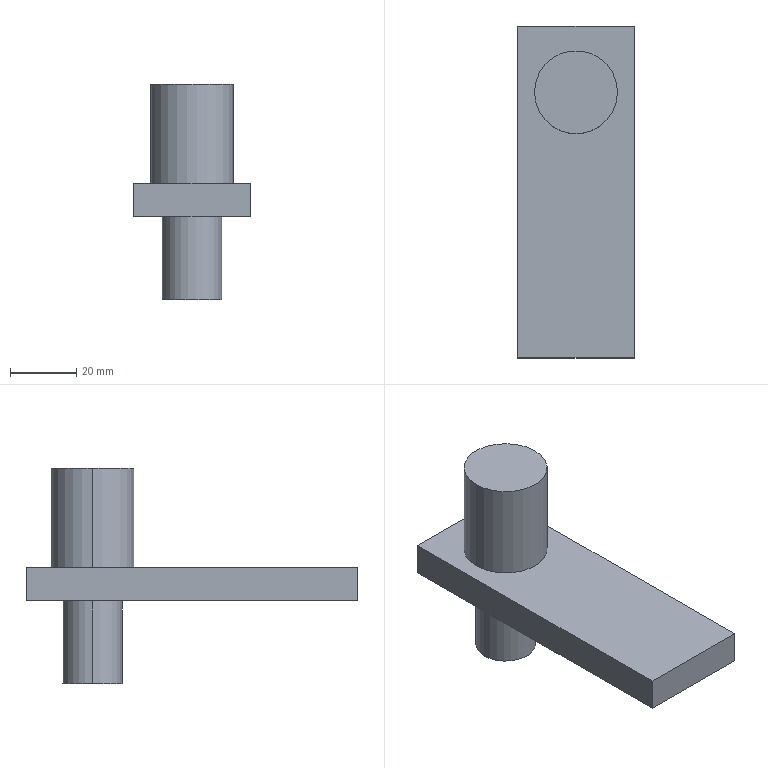Part | SolidWorks | features ICE 2, Extrusion 1 | 1 solid | 12 faces | box 35 x 100 x 65 mm | volume 56088 mm3 | plane 8 | cylinder 4 | commonest cylinder face diameters 18 x2 25 x2
STEP:
#1=CARTESIAN_POINT('',(-9.,30.,-25.));
#2=VERTEX_POINT('',#1);
#3=CARTESIAN_POINT('',(9.,30.,-25.));
#4=VERTEX_POINT('',#3);
#5=CARTESIAN_POINT('',(0.,30.,-25.));
#6=DIRECTION('',(0.,0.,-1.));
#7=DIRECTION('',(-1.,0.,0.));
#8=AXIS2_PLACEMENT_3D('',#5,#6,#7);
#9=CIRCLE('',#8,9.);
#10=EDGE_CURVE('',#2,#4,#9,.T.);
#11=ORIENTED_EDGE('',*,*,#10,.F.);
#12=CARTESIAN_POINT('',(-9.,30.,0.));
#13=VERTEX_POINT('',#12);
#14=CARTESIAN_POINT('',(-9.,30.,-25.));
#15=DIRECTION('',(0.,0.,1.));
#16=VECTOR('',#15,1000.);
#17=LINE('',#14,#16);
#18=EDGE_CURVE('',#2,#13,#17,.T.);
#19=ORIENTED_EDGE('',*,*,#18,.T.);
#20=CARTESIAN_POINT('',(9.,30.,0.));
#21=VERTEX_POINT('',#20);
#22=CARTESIAN_POINT('',(0.,30.,0.));
#23=DIRECTION('',(0.,0.,-1.));
#24=DIRECTION('',(-1.,0.,0.));
#25=AXIS2_PLACEMENT_3D('',#22,#23,#24);
#26=CIRCLE('',#25,9.);
#27=EDGE_CURVE('',#13,#21,#26,.T.);
#28=ORIENTED_EDGE('',*,*,#27,.T.);
#29=CARTESIAN_POINT('',(9.,30.,-25.));
#30=DIRECTION('',(0.,0.,1.));
#31=VECTOR('',#30,1000.);
#32=LINE('',#29,#31);
#33=EDGE_CURVE('',#4,#21,#32,.T.);
#34=ORIENTED_EDGE('',*,*,#33,.F.);
#35=EDGE_LOOP('',(#11,#19,#28,#34));
#36=FACE_OUTER_BOUND('',#35,.T.);
#37=CARTESIAN_POINT('',(0.,30.,-25.));
#38=DIRECTION('',(0.,0.,1.));
#39=DIRECTION('',(1.,0.,0.));
#40=AXIS2_PLACEMENT_3D('',#37,#38,#39);
#41=CYLINDRICAL_SURFACE('',#40,9.);
#42=ADVANCED_FACE('',(#36),#41,.T.);
#43=CARTESIAN_POINT('',(12.5,30.,40.));
#44=VERTEX_POINT('',#43);
#45=CARTESIAN_POINT('',(-12.5,30.,40.));
#46=VERTEX_POINT('',#45);
#47=CARTESIAN_POINT('',(0.,30.,40.));
#48=DIRECTION('',(0.,0.,1.));
#49=DIRECTION('',(1.,0.,0.));
#50=AXIS2_PLACEMENT_3D('',#47,#48,#49);
#51=CIRCLE('',#50,12.5);
#52=EDGE_CURVE('',#44,#46,#51,.T.);
#53=ORIENTED_EDGE('',*,*,#52,.F.);
#54=CARTESIAN_POINT('',(12.5,30.,10.));
#55=VERTEX_POINT('',#54);
#56=CARTESIAN_POINT('',(12.5,30.,40.));
#57=DIRECTION('',(0.,0.,-1.));
#58=VECTOR('',#57,1000.);
#59=LINE('',#56,#58);
#60=EDGE_CURVE('',#44,#55,#59,.T.);
#61=ORIENTED_EDGE('',*,*,#60,.T.);
#62=CARTESIAN_POINT('',(-12.5,30.,10.));
#63=VERTEX_POINT('',#62);
#64=CARTESIAN_POINT('',(0.,30.,10.));
#65=DIRECTION('',(0.,0.,1.));
#66=DIRECTION('',(-1.,0.,0.));
#67=AXIS2_PLACEMENT_3D('',#64,#65,#66);
#68=CIRCLE('',#67,12.5);
#69=EDGE_CURVE('',#55,#63,#68,.T.);
#70=ORIENTED_EDGE('',*,*,#69,.T.);
#71=CARTESIAN_POINT('',(-12.5,30.,40.));
#72=DIRECTION('',(0.,0.,-1.));
#73=VECTOR('',#72,1000.);
#74=LINE('',#71,#73);
#75=EDGE_CURVE('',#46,#63,#74,.T.);
#76=ORIENTED_EDGE('',*,*,#75,.F.);
#77=EDGE_LOOP('',(#53,#61,#70,#76));
#78=FACE_OUTER_BOUND('',#77,.T.);
#79=CARTESIAN_POINT('',(0.,30.,40.));
#80=DIRECTION('',(0.,0.,-1.));
#81=DIRECTION('',(-1.,0.,0.));
#82=AXIS2_PLACEMENT_3D('',#79,#80,#81);
#83=CYLINDRICAL_SURFACE('',#82,12.5);
#84=ADVANCED_FACE('',(#78),#83,.T.);
#85=CARTESIAN_POINT('',(17.5,-50.,0.));
#86=VERTEX_POINT('',#85);
#87=CARTESIAN_POINT('',(17.5,50.,0.));
#88=VERTEX_POINT('',#87);
#89=CARTESIAN_POINT('',(17.5,-50.,0.));
#90=DIRECTION('',(0.,1.,0.));
#91=VECTOR('',#90,1000.);
#92=LINE('',#89,#91);
#93=EDGE_CURVE('',#86,#88,#92,.T.);
#94=ORIENTED_EDGE('',*,*,#93,.T.);
#95=CARTESIAN_POINT('',(17.5,50.,10.));
#96=VERTEX_POINT('',#95);
#97=CARTESIAN_POINT('',(17.5,50.,10.));
#98=DIRECTION('',(0.,0.,-1.));
#99=VECTOR('',#98,1000.);
#100=LINE('',#97,#99);
#101=EDGE_CURVE('',#96,#88,#100,.T.);
#102=ORIENTED_EDGE('',*,*,#101,.F.);
#103=CARTESIAN_POINT('',(17.5,-50.,10.));
#104=VERTEX_POINT('',#103);
#105=CARTESIAN_POINT('',(17.5,-50.,10.));
#106=DIRECTION('',(0.,1.,0.));
#107=VECTOR('',#106,1000.);
#108=LINE('',#105,#107);
#109=EDGE_CURVE('',#104,#96,#108,.T.);
#110=ORIENTED_EDGE('',*,*,#109,.F.);
#111=CARTESIAN_POINT('',(17.5,-50.,10.));
#112=DIRECTION('',(0.,0.,-1.));
#113=VECTOR('',#112,1000.);
#114=LINE('',#111,#113);
#115=EDGE_CURVE('',#104,#86,#114,.T.);
#116=ORIENTED_EDGE('',*,*,#115,.T.);
#117=EDGE_LOOP('',(#94,#102,#110,#116));
#118=FACE_OUTER_BOUND('',#117,.T.);
#119=CARTESIAN_POINT('',(17.5,-50.,10.));
#120=DIRECTION('',(-1.,0.,0.));
#121=DIRECTION('',(0.,0.,1.));
#122=AXIS2_PLACEMENT_3D('',#119,#120,#121);
#123=PLANE('',#122);
#124=ADVANCED_FACE('',(#118),#123,.F.);
#125=CARTESIAN_POINT('',(-17.5,50.,0.));
#126=VERTEX_POINT('',#125);
#127=CARTESIAN_POINT('',(-17.5,50.,0.));
#128=DIRECTION('',(-1.,0.,0.));
#129=VECTOR('',#128,1000.);
#130=LINE('',#127,#129);
#131=EDGE_CURVE('',#88,#126,#130,.T.);
#132=ORIENTED_EDGE('',*,*,#131,.T.);
#133=CARTESIAN_POINT('',(-17.5,50.,10.));
#134=VERTEX_POINT('',#133);
#135=CARTESIAN_POINT('',(-17.5,50.,10.));
#136=DIRECTION('',(0.,0.,-1.));
#137=VECTOR('',#136,1000.);
#138=LINE('',#135,#137);
#139=EDGE_CURVE('',#134,#126,#138,.T.);
#140=ORIENTED_EDGE('',*,*,#139,.F.);
#141=CARTESIAN_POINT('',(-17.5,50.,10.));
#142=DIRECTION('',(-1.,0.,0.));
#143=VECTOR('',#142,1000.);
#144=LINE('',#141,#143);
#145=EDGE_CURVE('',#96,#134,#144,.T.);
#146=ORIENTED_EDGE('',*,*,#145,.F.);
#147=ORIENTED_EDGE('',*,*,#101,.T.);
#148=EDGE_LOOP('',(#132,#140,#146,#147));
#149=FACE_OUTER_BOUND('',#148,.T.);
#150=CARTESIAN_POINT('',(-17.5,50.,10.));
#151=DIRECTION('',(0.,-1.,0.));
#152=DIRECTION('',(0.,0.,-1.));
#153=AXIS2_PLACEMENT_3D('',#150,#151,#152);
#154=PLANE('',#153);
#155=ADVANCED_FACE('',(#149),#154,.F.);
#156=CARTESIAN_POINT('',(-17.5,-50.,0.));
#157=VERTEX_POINT('',#156);
#158=CARTESIAN_POINT('',(-17.5,-50.,0.));
#159=DIRECTION('',(0.,-1.,0.));
#160=VECTOR('',#159,1000.);
#161=LINE('',#158,#160);
#162=EDGE_CURVE('',#126,#157,#161,.T.);
#163=ORIENTED_EDGE('',*,*,#162,.T.);
#164=CARTESIAN_POINT('',(-17.5,-50.,10.));
#165=VERTEX_POINT('',#164);
#166=CARTESIAN_POINT('',(-17.5,-50.,10.));
#167=DIRECTION('',(0.,0.,-1.));
#168=VECTOR('',#167,1000.);
#169=LINE('',#166,#168);
#170=EDGE_CURVE('',#165,#157,#169,.T.);
#171=ORIENTED_EDGE('',*,*,#170,.F.);
#172=CARTESIAN_POINT('',(-17.5,-50.,10.));
#173=DIRECTION('',(0.,-1.,0.));
#174=VECTOR('',#173,1000.);
#175=LINE('',#172,#174);
#176=EDGE_CURVE('',#134,#165,#175,.T.);
#177=ORIENTED_EDGE('',*,*,#176,.F.);
#178=ORIENTED_EDGE('',*,*,#139,.T.);
#179=EDGE_LOOP('',(#163,#171,#177,#178));
#180=FACE_OUTER_BOUND('',#179,.T.);
#181=CARTESIAN_POINT('',(-17.5,-50.,10.));
#182=DIRECTION('',(1.,0.,0.));
#183=DIRECTION('',(0.,0.,-1.));
#184=AXIS2_PLACEMENT_3D('',#181,#182,#183);
#185=PLANE('',#184);
#186=ADVANCED_FACE('',(#180),#185,.F.);
#187=CARTESIAN_POINT('',(-17.5,-50.,0.));
#188=DIRECTION('',(1.,0.,0.));
#189=VECTOR('',#188,1000.);
#190=LINE('',#187,#189);
#191=EDGE_CURVE('',#157,#86,#190,.T.);
#192=ORIENTED_EDGE('',*,*,#191,.T.);
#193=ORIENTED_EDGE('',*,*,#115,.F.);
#194=CARTESIAN_POINT('',(-17.5,-50.,10.));
#195=DIRECTION('',(1.,0.,0.));
#196=VECTOR('',#195,1000.);
#197=LINE('',#194,#196);
#198=EDGE_CURVE('',#165,#104,#197,.T.);
#199=ORIENTED_EDGE('',*,*,#198,.F.);
#200=ORIENTED_EDGE('',*,*,#170,.T.);
#201=EDGE_LOOP('',(#192,#193,#199,#200));
#202=FACE_OUTER_BOUND('',#201,.T.);
#203=CARTESIAN_POINT('',(-17.5,-50.,10.));
#204=DIRECTION('',(0.,1.,0.));
#205=DIRECTION('',(0.,0.,1.));
#206=AXIS2_PLACEMENT_3D('',#203,#204,#205);
#207=PLANE('',#206);
#208=ADVANCED_FACE('',(#202),#207,.F.);
#209=CARTESIAN_POINT('',(0.,30.,10.));
#210=DIRECTION('',(0.,0.,1.));
#211=DIRECTION('',(-1.,0.,0.));
#212=AXIS2_PLACEMENT_3D('',#209,#210,#211);
#213=CIRCLE('',#212,12.5);
#214=EDGE_CURVE('',#63,#55,#213,.T.);
#215=ORIENTED_EDGE('',*,*,#214,.F.);
#216=ORIENTED_EDGE('',*,*,#69,.F.);
#217=EDGE_LOOP('',(#215,#216));
#218=FACE_BOUND('',#217,.T.);
#219=ORIENTED_EDGE('',*,*,#109,.T.);
#220=ORIENTED_EDGE('',*,*,#145,.T.);
#221=ORIENTED_EDGE('',*,*,#176,.T.);
#222=ORIENTED_EDGE('',*,*,#198,.T.);
#223=EDGE_LOOP('',(#219,#220,#221,#222));
#224=FACE_OUTER_BOUND('',#223,.T.);
#225=CARTESIAN_POINT('',(0.,0.,10.));
#226=DIRECTION('',(0.,0.,-1.));
#227=DIRECTION('',(-1.,0.,0.));
#228=AXIS2_PLACEMENT_3D('',#225,#226,#227);
#229=PLANE('',#228);
#230=ADVANCED_FACE('',(#218,#224),#229,.F.);
#231=CARTESIAN_POINT('',(0.,30.,0.));
#232=DIRECTION('',(0.,0.,-1.));
#233=DIRECTION('',(-1.,0.,0.));
#234=AXIS2_PLACEMENT_3D('',#231,#232,#233);
#235=CIRCLE('',#234,9.);
#236=EDGE_CURVE('',#21,#13,#235,.T.);
#237=ORIENTED_EDGE('',*,*,#236,.F.);
#238=ORIENTED_EDGE('',*,*,#27,.F.);
#239=EDGE_LOOP('',(#237,#238));
#240=FACE_BOUND('',#239,.T.);
#241=ORIENTED_EDGE('',*,*,#93,.F.);
#242=ORIENTED_EDGE('',*,*,#191,.F.);
#243=ORIENTED_EDGE('',*,*,#162,.F.);
#244=ORIENTED_EDGE('',*,*,#131,.F.);
#245=EDGE_LOOP('',(#241,#242,#243,#244));
#246=FACE_OUTER_BOUND('',#245,.T.);
#247=CARTESIAN_POINT('',(0.,0.,0.));
#248=DIRECTION('',(0.,0.,-1.));
#249=DIRECTION('',(-1.,0.,0.));
#250=AXIS2_PLACEMENT_3D('',#247,#248,#249);
#251=PLANE('',#250);
#252=ADVANCED_FACE('',(#240,#246),#251,.T.);
#253=ORIENTED_EDGE('',*,*,#60,.F.);
#254=CARTESIAN_POINT('',(0.,30.,40.));
#255=DIRECTION('',(0.,0.,1.));
#256=DIRECTION('',(1.,0.,0.));
#257=AXIS2_PLACEMENT_3D('',#254,#255,#256);
#258=CIRCLE('',#257,12.5);
#259=EDGE_CURVE('',#46,#44,#258,.T.);
#260=ORIENTED_EDGE('',*,*,#259,.F.);
#261=ORIENTED_EDGE('',*,*,#75,.T.);
#262=ORIENTED_EDGE('',*,*,#214,.T.);
#263=EDGE_LOOP('',(#253,#260,#261,#262));
#264=FACE_OUTER_BOUND('',#263,.T.);
#265=CARTESIAN_POINT('',(0.,30.,40.));
#266=DIRECTION('',(0.,0.,-1.));
#267=DIRECTION('',(-1.,0.,0.));
#268=AXIS2_PLACEMENT_3D('',#265,#266,#267);
#269=CYLINDRICAL_SURFACE('',#268,12.5);
#270=ADVANCED_FACE('',(#264),#269,.T.);
#271=ORIENTED_EDGE('',*,*,#259,.T.);
#272=ORIENTED_EDGE('',*,*,#52,.T.);
#273=EDGE_LOOP('',(#271,#272));
#274=FACE_OUTER_BOUND('',#273,.T.);
#275=CARTESIAN_POINT('',(0.,30.,40.));
#276=DIRECTION('',(0.,0.,1.));
#277=DIRECTION('',(1.,0.,0.));
#278=AXIS2_PLACEMENT_3D('',#275,#276,#277);
#279=PLANE('',#278);
#280=ADVANCED_FACE('',(#274),#279,.T.);
#281=ORIENTED_EDGE('',*,*,#18,.F.);
#282=CARTESIAN_POINT('',(0.,30.,-25.));
#283=DIRECTION('',(0.,0.,-1.));
#284=DIRECTION('',(-1.,0.,0.));
#285=AXIS2_PLACEMENT_3D('',#282,#283,#284);
#286=CIRCLE('',#285,9.);
#287=EDGE_CURVE('',#4,#2,#286,.T.);
#288=ORIENTED_EDGE('',*,*,#287,.F.);
#289=ORIENTED_EDGE('',*,*,#33,.T.);
#290=ORIENTED_EDGE('',*,*,#236,.T.);
#291=EDGE_LOOP('',(#281,#288,#289,#290));
#292=FACE_OUTER_BOUND('',#291,.T.);
#293=CARTESIAN_POINT('',(0.,30.,-25.));
#294=DIRECTION('',(0.,0.,1.));
#295=DIRECTION('',(1.,0.,0.));
#296=AXIS2_PLACEMENT_3D('',#293,#294,#295);
#297=CYLINDRICAL_SURFACE('',#296,9.);
#298=ADVANCED_FACE('',(#292),#297,.T.);
#299=ORIENTED_EDGE('',*,*,#287,.T.);
#300=ORIENTED_EDGE('',*,*,#10,.T.);
#301=EDGE_LOOP('',(#299,#300));
#302=FACE_OUTER_BOUND('',#301,.T.);
#303=CARTESIAN_POINT('',(0.,30.,-25.));
#304=DIRECTION('',(0.,0.,-1.));
#305=DIRECTION('',(-1.,0.,0.));
#306=AXIS2_PLACEMENT_3D('',#303,#304,#305);
#307=PLANE('',#306);
#308=ADVANCED_FACE('',(#302),#307,.T.);
#309=CLOSED_SHELL('',(#42,#84,#124,#155,#186,#208,#230,#252,#270,#280,#298,#308));
#310=MANIFOLD_SOLID_BREP('',#309);
#311=CARTESIAN_POINT('',(0.,0.,0.));
#312=DIRECTION('',(0.,0.,1.));
#313=DIRECTION('',(1.,0.,0.));
#314=AXIS2_PLACEMENT_3D('',#311,#312,#313);
#315=(LENGTH_UNIT()NAMED_UNIT(*)SI_UNIT(.MILLI.,.METRE.));
#316=UNCERTAINTY_MEASURE_WITH_UNIT(LENGTH_MEASURE(0.00001),#315,'','');
#317=(NAMED_UNIT(*)PLANE_ANGLE_UNIT()SI_UNIT($,.RADIAN.));
#318=(NAMED_UNIT(*)SI_UNIT($,.STERADIAN.)SOLID_ANGLE_UNIT());
#319=(GEOMETRIC_REPRESENTATION_CONTEXT(3)GLOBAL_UNCERTAINTY_ASSIGNED_CONTEXT((#316))GLOBAL_UNIT_ASSIGNED_CONTEXT((#315,#317,#318))REPRESENTATION_CONTEXT('',''));
#320=ADVANCED_BREP_SHAPE_REPRESENTATION('',(#310,#314),#319);